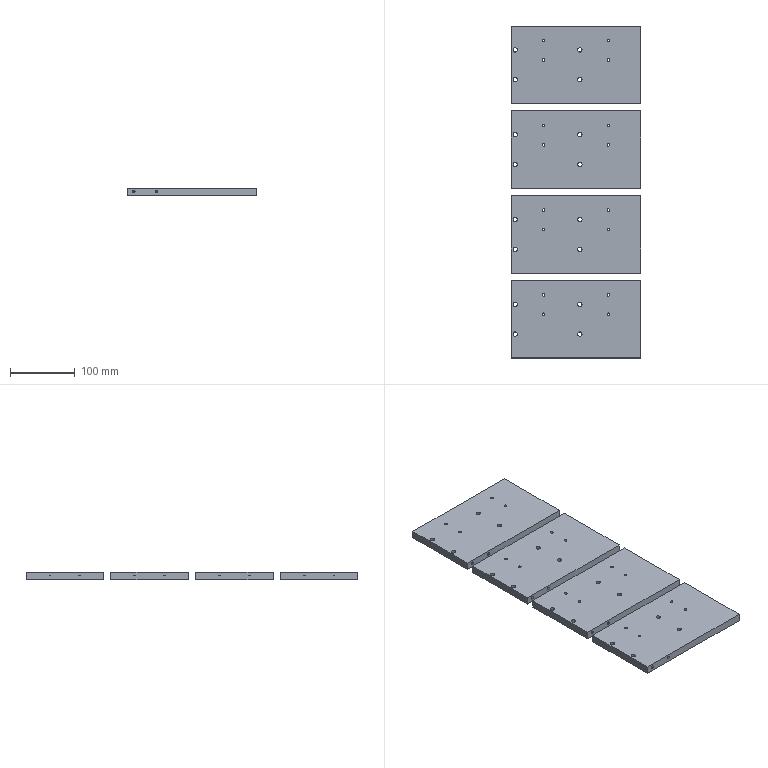Part | 4 solids | 104 faces | box 200 x 513 x 12 mm | volume 1134668 mm3 | cylinder 56 | plane 40 | cone 8 | commonest cylinder face diameters 4.134 x24 6.6 x16 11 x16